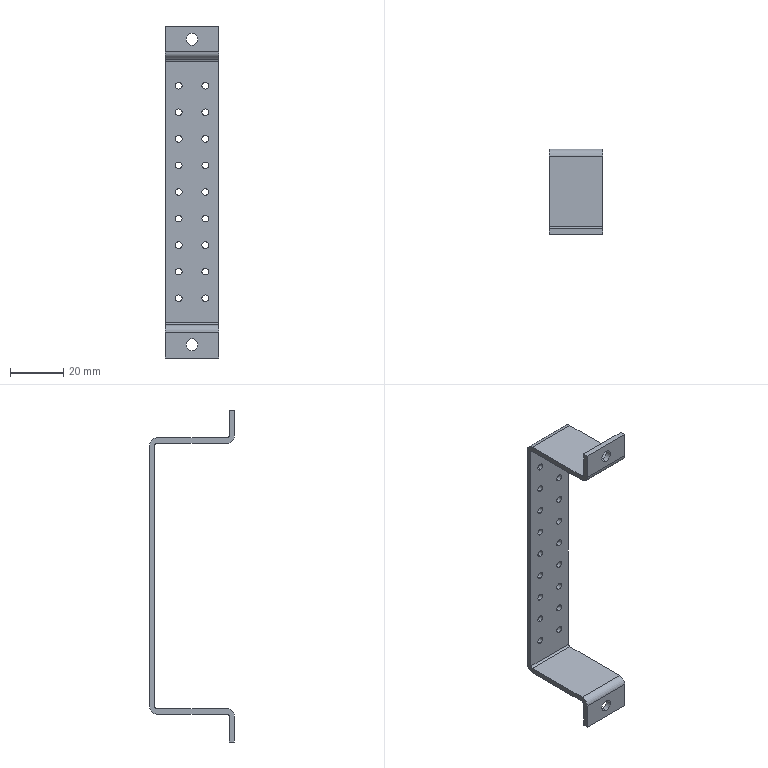Part | SolidWorks | features BaseBody 1 | 1 solid | 62 faces | box 20 x 32 x 125 mm | volume 7040 mm3 | cylinder 48 | plane 14 | commonest cylinder face diameters 2.5 x36 1.473 x4 4.5 x4 5.473 x4